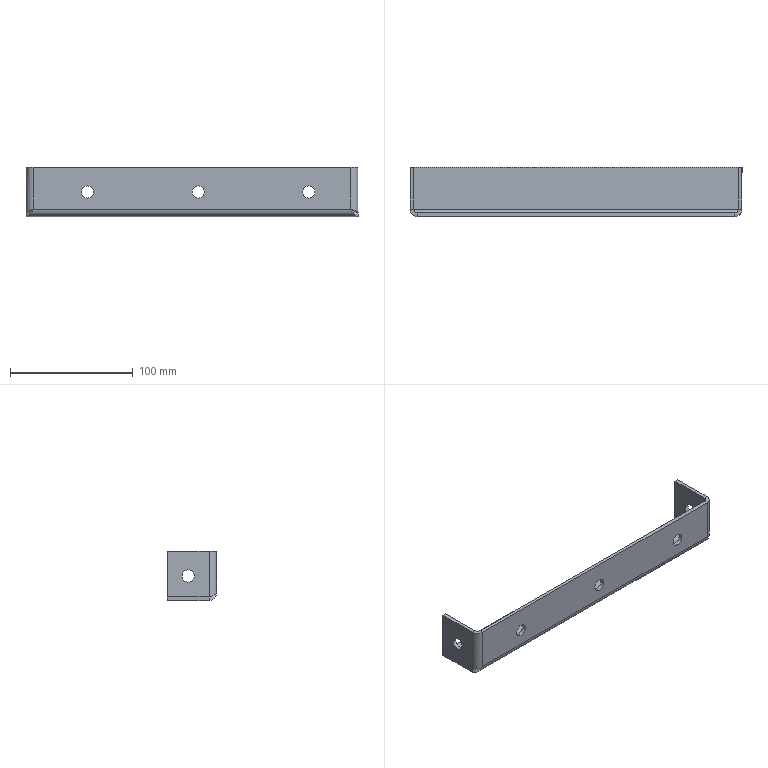Part | SolidWorks | features CornerFeat 1, EdgeFlange 1, FlatPattern 1, ICE 1, SMBaseFlange 1, SheetMetal 1 | 1 solid | 40 faces | box 270 x 40 x 40 mm | volume 67307 mm3 | plane 20 | cylinder 16 | spline 4 | commonest cylinder face diameters 10 x10 6 x3 12 x3
STEP:
#1=CARTESIAN_POINT('',(132.,28.,0.));
#2=VERTEX_POINT('',#1);
#3=CARTESIAN_POINT('',(132.,18.,0.));
#4=VERTEX_POINT('',#3);
#5=CARTESIAN_POINT('',(132.,23.,0.));
#6=DIRECTION('',(-1.,0.,0.));
#7=DIRECTION('',(0.,-1.,0.));
#8=AXIS2_PLACEMENT_3D('',#5,#6,#7);
#9=CIRCLE('',#8,5.);
#10=EDGE_CURVE('',#2,#4,#9,.T.);
#11=ORIENTED_EDGE('',*,*,#10,.T.);
#12=CARTESIAN_POINT('',(135.,18.,0.));
#13=VERTEX_POINT('',#12);
#14=CARTESIAN_POINT('',(-239.,18.,0.));
#15=DIRECTION('',(1.,0.,0.));
#16=VECTOR('',#15,1000.);
#17=LINE('',#14,#16);
#18=EDGE_CURVE('',#4,#13,#17,.T.);
#19=ORIENTED_EDGE('',*,*,#18,.T.);
#20=CARTESIAN_POINT('',(135.,28.,0.));
#21=VERTEX_POINT('',#20);
#22=CARTESIAN_POINT('',(135.,23.,0.));
#23=DIRECTION('',(1.,0.,0.));
#24=DIRECTION('',(0.,1.,0.));
#25=AXIS2_PLACEMENT_3D('',#22,#23,#24);
#26=CIRCLE('',#25,5.);
#27=EDGE_CURVE('',#13,#21,#26,.T.);
#28=ORIENTED_EDGE('',*,*,#27,.T.);
#29=CARTESIAN_POINT('',(-239.,28.,0.));
#30=DIRECTION('',(1.,0.,0.));
#31=VECTOR('',#30,1000.);
#32=LINE('',#29,#31);
#33=EDGE_CURVE('',#2,#21,#32,.T.);
#34=ORIENTED_EDGE('',*,*,#33,.F.);
#35=EDGE_LOOP('',(#11,#19,#28,#34));
#36=FACE_OUTER_BOUND('',#35,.T.);
#37=CARTESIAN_POINT('',(-239.,23.,0.));
#38=DIRECTION('',(1.,0.,0.));
#39=DIRECTION('',(0.,1.,0.));
#40=AXIS2_PLACEMENT_3D('',#37,#38,#39);
#41=CYLINDRICAL_SURFACE('',#40,5.);
#42=ADVANCED_FACE('',(#36),#41,.F.);
#43=CARTESIAN_POINT('',(-135.,18.,0.));
#44=VERTEX_POINT('',#43);
#45=CARTESIAN_POINT('',(-135.,28.,0.));
#46=VERTEX_POINT('',#45);
#47=CARTESIAN_POINT('',(-135.,23.,0.));
#48=DIRECTION('',(1.,0.,0.));
#49=DIRECTION('',(0.,1.,0.));
#50=AXIS2_PLACEMENT_3D('',#47,#48,#49);
#51=CIRCLE('',#50,5.);
#52=EDGE_CURVE('',#44,#46,#51,.T.);
#53=ORIENTED_EDGE('',*,*,#52,.F.);
#54=CARTESIAN_POINT('',(-132.,18.,0.));
#55=VERTEX_POINT('',#54);
#56=CARTESIAN_POINT('',(-239.,18.,0.));
#57=DIRECTION('',(1.,0.,0.));
#58=VECTOR('',#57,1000.);
#59=LINE('',#56,#58);
#60=EDGE_CURVE('',#44,#55,#59,.T.);
#61=ORIENTED_EDGE('',*,*,#60,.T.);
#62=CARTESIAN_POINT('',(-132.,28.,0.));
#63=VERTEX_POINT('',#62);
#64=CARTESIAN_POINT('',(-132.,23.,0.));
#65=DIRECTION('',(1.,0.,0.));
#66=DIRECTION('',(0.,1.,0.));
#67=AXIS2_PLACEMENT_3D('',#64,#65,#66);
#68=CIRCLE('',#67,5.);
#69=EDGE_CURVE('',#55,#63,#68,.T.);
#70=ORIENTED_EDGE('',*,*,#69,.T.);
#71=CARTESIAN_POINT('',(-239.,28.,0.));
#72=DIRECTION('',(1.,0.,0.));
#73=VECTOR('',#72,1000.);
#74=LINE('',#71,#73);
#75=EDGE_CURVE('',#46,#63,#74,.T.);
#76=ORIENTED_EDGE('',*,*,#75,.F.);
#77=EDGE_LOOP('',(#53,#61,#70,#76));
#78=FACE_OUTER_BOUND('',#77,.T.);
#79=CARTESIAN_POINT('',(-239.,23.,0.));
#80=DIRECTION('',(1.,0.,0.));
#81=DIRECTION('',(0.,1.,0.));
#82=AXIS2_PLACEMENT_3D('',#79,#80,#81);
#83=CYLINDRICAL_SURFACE('',#82,5.);
#84=ADVANCED_FACE('',(#78),#83,.F.);
#85=CARTESIAN_POINT('',(95.,3.,-5.));
#86=VERTEX_POINT('',#85);
#87=CARTESIAN_POINT('',(95.,3.,5.));
#88=VERTEX_POINT('',#87);
#89=CARTESIAN_POINT('',(95.,3.,0.));
#90=DIRECTION('',(0.,1.,0.));
#91=DIRECTION('',(0.,0.,1.));
#92=AXIS2_PLACEMENT_3D('',#89,#90,#91);
#93=CIRCLE('',#92,5.);
#94=EDGE_CURVE('',#86,#88,#93,.T.);
#95=ORIENTED_EDGE('',*,*,#94,.T.);
#96=CARTESIAN_POINT('',(95.,0.,5.));
#97=VERTEX_POINT('',#96);
#98=CARTESIAN_POINT('',(95.,3.,5.));
#99=DIRECTION('',(0.,-1.,0.));
#100=VECTOR('',#99,1000.);
#101=LINE('',#98,#100);
#102=EDGE_CURVE('',#88,#97,#101,.T.);
#103=ORIENTED_EDGE('',*,*,#102,.T.);
#104=CARTESIAN_POINT('',(95.,0.,-5.));
#105=VERTEX_POINT('',#104);
#106=CARTESIAN_POINT('',(95.,0.,0.));
#107=DIRECTION('',(0.,1.,0.));
#108=DIRECTION('',(0.,0.,1.));
#109=AXIS2_PLACEMENT_3D('',#106,#107,#108);
#110=CIRCLE('',#109,5.);
#111=EDGE_CURVE('',#105,#97,#110,.T.);
#112=ORIENTED_EDGE('',*,*,#111,.F.);
#113=CARTESIAN_POINT('',(95.,3.,-5.));
#114=DIRECTION('',(0.,-1.,0.));
#115=VECTOR('',#114,1000.);
#116=LINE('',#113,#115);
#117=EDGE_CURVE('',#86,#105,#116,.T.);
#118=ORIENTED_EDGE('',*,*,#117,.F.);
#119=EDGE_LOOP('',(#95,#103,#112,#118));
#120=FACE_OUTER_BOUND('',#119,.T.);
#121=CARTESIAN_POINT('',(95.,3.,0.));
#122=DIRECTION('',(0.,-1.,0.));
#123=DIRECTION('',(0.,0.,-1.));
#124=AXIS2_PLACEMENT_3D('',#121,#122,#123);
#125=CYLINDRICAL_SURFACE('',#124,5.);
#126=ADVANCED_FACE('',(#120),#125,.F.);
#127=CARTESIAN_POINT('',(5.,3.,-5.));
#128=VERTEX_POINT('',#127);
#129=CARTESIAN_POINT('',(5.,3.,5.));
#130=VERTEX_POINT('',#129);
#131=CARTESIAN_POINT('',(5.,3.,0.));
#132=DIRECTION('',(0.,1.,0.));
#133=DIRECTION('',(0.,0.,1.));
#134=AXIS2_PLACEMENT_3D('',#131,#132,#133);
#135=CIRCLE('',#134,5.);
#136=EDGE_CURVE('',#128,#130,#135,.T.);
#137=ORIENTED_EDGE('',*,*,#136,.T.);
#138=CARTESIAN_POINT('',(5.,0.,5.));
#139=VERTEX_POINT('',#138);
#140=CARTESIAN_POINT('',(5.,3.,5.));
#141=DIRECTION('',(0.,-1.,0.));
#142=VECTOR('',#141,1000.);
#143=LINE('',#140,#142);
#144=EDGE_CURVE('',#130,#139,#143,.T.);
#145=ORIENTED_EDGE('',*,*,#144,.T.);
#146=CARTESIAN_POINT('',(5.,0.,-5.));
#147=VERTEX_POINT('',#146);
#148=CARTESIAN_POINT('',(5.,0.,0.));
#149=DIRECTION('',(0.,1.,0.));
#150=DIRECTION('',(0.,0.,1.));
#151=AXIS2_PLACEMENT_3D('',#148,#149,#150);
#152=CIRCLE('',#151,5.);
#153=EDGE_CURVE('',#147,#139,#152,.T.);
#154=ORIENTED_EDGE('',*,*,#153,.F.);
#155=CARTESIAN_POINT('',(5.,3.,-5.));
#156=DIRECTION('',(0.,-1.,0.));
#157=VECTOR('',#156,1000.);
#158=LINE('',#155,#157);
#159=EDGE_CURVE('',#128,#147,#158,.T.);
#160=ORIENTED_EDGE('',*,*,#159,.F.);
#161=EDGE_LOOP('',(#137,#145,#154,#160));
#162=FACE_OUTER_BOUND('',#161,.T.);
#163=CARTESIAN_POINT('',(5.,3.,0.));
#164=DIRECTION('',(0.,-1.,0.));
#165=DIRECTION('',(0.,0.,-1.));
#166=AXIS2_PLACEMENT_3D('',#163,#164,#165);
#167=CYLINDRICAL_SURFACE('',#166,5.);
#168=ADVANCED_FACE('',(#162),#167,.F.);
#169=CARTESIAN_POINT('',(-85.,3.,-5.));
#170=VERTEX_POINT('',#169);
#171=CARTESIAN_POINT('',(-85.,3.,5.));
#172=VERTEX_POINT('',#171);
#173=CARTESIAN_POINT('',(-85.,3.,0.));
#174=DIRECTION('',(0.,1.,0.));
#175=DIRECTION('',(0.,0.,1.));
#176=AXIS2_PLACEMENT_3D('',#173,#174,#175);
#177=CIRCLE('',#176,5.);
#178=EDGE_CURVE('',#170,#172,#177,.T.);
#179=ORIENTED_EDGE('',*,*,#178,.T.);
#180=CARTESIAN_POINT('',(-85.,0.,5.));
#181=VERTEX_POINT('',#180);
#182=CARTESIAN_POINT('',(-85.,3.,5.));
#183=DIRECTION('',(0.,-1.,0.));
#184=VECTOR('',#183,1000.);
#185=LINE('',#182,#184);
#186=EDGE_CURVE('',#172,#181,#185,.T.);
#187=ORIENTED_EDGE('',*,*,#186,.T.);
#188=CARTESIAN_POINT('',(-85.,0.,-5.));
#189=VERTEX_POINT('',#188);
#190=CARTESIAN_POINT('',(-85.,0.,0.));
#191=DIRECTION('',(0.,1.,0.));
#192=DIRECTION('',(0.,0.,1.));
#193=AXIS2_PLACEMENT_3D('',#190,#191,#192);
#194=CIRCLE('',#193,5.);
#195=EDGE_CURVE('',#189,#181,#194,.T.);
#196=ORIENTED_EDGE('',*,*,#195,.F.);
#197=CARTESIAN_POINT('',(-85.,3.,-5.));
#198=DIRECTION('',(0.,-1.,0.));
#199=VECTOR('',#198,1000.);
#200=LINE('',#197,#199);
#201=EDGE_CURVE('',#170,#189,#200,.T.);
#202=ORIENTED_EDGE('',*,*,#201,.F.);
#203=EDGE_LOOP('',(#179,#187,#196,#202));
#204=FACE_OUTER_BOUND('',#203,.T.);
#205=CARTESIAN_POINT('',(-85.,3.,0.));
#206=DIRECTION('',(0.,-1.,0.));
#207=DIRECTION('',(0.,0.,-1.));
#208=AXIS2_PLACEMENT_3D('',#205,#206,#207);
#209=CYLINDRICAL_SURFACE('',#208,5.);
#210=ADVANCED_FACE('',(#204),#209,.F.);
#211=ORIENTED_EDGE('',*,*,#136,.F.);
#212=CARTESIAN_POINT('',(5.,3.,0.));
#213=DIRECTION('',(0.,1.,0.));
#214=DIRECTION('',(0.,0.,1.));
#215=AXIS2_PLACEMENT_3D('',#212,#213,#214);
#216=CIRCLE('',#215,5.);
#217=EDGE_CURVE('',#130,#128,#216,.T.);
#218=ORIENTED_EDGE('',*,*,#217,.F.);
#219=EDGE_LOOP('',(#211,#218));
#220=FACE_BOUND('',#219,.T.);
#221=ORIENTED_EDGE('',*,*,#178,.F.);
#222=CARTESIAN_POINT('',(-85.,3.,0.));
#223=DIRECTION('',(0.,1.,0.));
#224=DIRECTION('',(0.,0.,1.));
#225=AXIS2_PLACEMENT_3D('',#222,#223,#224);
#226=CIRCLE('',#225,5.);
#227=EDGE_CURVE('',#172,#170,#226,.T.);
#228=ORIENTED_EDGE('',*,*,#227,.F.);
#229=EDGE_LOOP('',(#221,#228));
#230=FACE_BOUND('',#229,.T.);
#231=ORIENTED_EDGE('',*,*,#94,.F.);
#232=CARTESIAN_POINT('',(95.,3.,0.));
#233=DIRECTION('',(0.,1.,0.));
#234=DIRECTION('',(0.,0.,1.));
#235=AXIS2_PLACEMENT_3D('',#232,#233,#234);
#236=CIRCLE('',#235,5.);
#237=EDGE_CURVE('',#88,#86,#236,.T.);
#238=ORIENTED_EDGE('',*,*,#237,.F.);
#239=EDGE_LOOP('',(#231,#238));
#240=FACE_BOUND('',#239,.T.);
#241=CARTESIAN_POINT('',(-129.,3.,-14.));
#242=VERTEX_POINT('',#241);
#243=CARTESIAN_POINT('',(129.,3.,-14.));
#244=VERTEX_POINT('',#243);
#245=CARTESIAN_POINT('',(-131.293,3.,-14.));
#246=DIRECTION('',(1.,0.,0.));
#247=VECTOR('',#246,1000.);
#248=LINE('',#245,#247);
#249=EDGE_CURVE('',#242,#244,#248,.T.);
#250=ORIENTED_EDGE('',*,*,#249,.F.);
#251=CARTESIAN_POINT('',(-129.,3.,20.));
#252=VERTEX_POINT('',#251);
#253=CARTESIAN_POINT('',(-129.,3.,20.));
#254=DIRECTION('',(0.,0.,-1.));
#255=VECTOR('',#254,1000.);
#256=LINE('',#253,#255);
#257=EDGE_CURVE('',#252,#242,#256,.T.);
#258=ORIENTED_EDGE('',*,*,#257,.F.);
#259=CARTESIAN_POINT('',(129.,3.,20.));
#260=VERTEX_POINT('',#259);
#261=CARTESIAN_POINT('',(-135.,3.,20.));
#262=DIRECTION('',(1.,0.,0.));
#263=VECTOR('',#262,1000.);
#264=LINE('',#261,#263);
#265=EDGE_CURVE('',#252,#260,#264,.T.);
#266=ORIENTED_EDGE('',*,*,#265,.T.);
#267=CARTESIAN_POINT('',(129.,3.,-16.293));
#268=DIRECTION('',(0.,0.,1.));
#269=VECTOR('',#268,1000.);
#270=LINE('',#267,#269);
#271=EDGE_CURVE('',#244,#260,#270,.T.);
#272=ORIENTED_EDGE('',*,*,#271,.F.);
#273=EDGE_LOOP('',(#250,#258,#266,#272));
#274=FACE_OUTER_BOUND('',#273,.T.);
#275=CARTESIAN_POINT('',(0.,3.,0.));
#276=DIRECTION('',(0.,1.,0.));
#277=DIRECTION('',(0.,0.,1.));
#278=AXIS2_PLACEMENT_3D('',#275,#276,#277);
#279=PLANE('',#278);
#280=ADVANCED_FACE('',(#220,#230,#240,#274),#279,.T.);
#281=ORIENTED_EDGE('',*,*,#111,.T.);
#282=CARTESIAN_POINT('',(95.,0.,0.));
#283=DIRECTION('',(0.,1.,0.));
#284=DIRECTION('',(0.,0.,1.));
#285=AXIS2_PLACEMENT_3D('',#282,#283,#284);
#286=CIRCLE('',#285,5.);
#287=EDGE_CURVE('',#97,#105,#286,.T.);
#288=ORIENTED_EDGE('',*,*,#287,.T.);
#289=EDGE_LOOP('',(#281,#288));
#290=FACE_BOUND('',#289,.T.);
#291=ORIENTED_EDGE('',*,*,#153,.T.);
#292=CARTESIAN_POINT('',(5.,0.,0.));
#293=DIRECTION('',(0.,1.,0.));
#294=DIRECTION('',(0.,0.,1.));
#295=AXIS2_PLACEMENT_3D('',#292,#293,#294);
#296=CIRCLE('',#295,5.);
#297=EDGE_CURVE('',#139,#147,#296,.T.);
#298=ORIENTED_EDGE('',*,*,#297,.T.);
#299=EDGE_LOOP('',(#291,#298));
#300=FACE_BOUND('',#299,.T.);
#301=ORIENTED_EDGE('',*,*,#195,.T.);
#302=CARTESIAN_POINT('',(-85.,0.,0.));
#303=DIRECTION('',(0.,1.,0.));
#304=DIRECTION('',(0.,0.,1.));
#305=AXIS2_PLACEMENT_3D('',#302,#303,#304);
#306=CIRCLE('',#305,5.);
#307=EDGE_CURVE('',#181,#189,#306,.T.);
#308=ORIENTED_EDGE('',*,*,#307,.T.);
#309=EDGE_LOOP('',(#301,#308));
#310=FACE_BOUND('',#309,.T.);
#311=CARTESIAN_POINT('',(-129.,0.,20.));
#312=VERTEX_POINT('',#311);
#313=CARTESIAN_POINT('',(-129.,0.,-14.));
#314=VERTEX_POINT('',#313);
#315=CARTESIAN_POINT('',(-129.,0.,20.));
#316=DIRECTION('',(0.,0.,-1.));
#317=VECTOR('',#316,1000.);
#318=LINE('',#315,#317);
#319=EDGE_CURVE('',#312,#314,#318,.T.);
#320=ORIENTED_EDGE('',*,*,#319,.T.);
#321=CARTESIAN_POINT('',(129.,0.,-14.));
#322=VERTEX_POINT('',#321);
#323=CARTESIAN_POINT('',(-131.293,0.,-14.));
#324=DIRECTION('',(1.,0.,0.));
#325=VECTOR('',#324,1000.);
#326=LINE('',#323,#325);
#327=EDGE_CURVE('',#314,#322,#326,.T.);
#328=ORIENTED_EDGE('',*,*,#327,.T.);
#329=CARTESIAN_POINT('',(129.,0.,20.));
#330=VERTEX_POINT('',#329);
#331=CARTESIAN_POINT('',(129.,0.,-16.293));
#332=DIRECTION('',(0.,0.,1.));
#333=VECTOR('',#332,1000.);
#334=LINE('',#331,#333);
#335=EDGE_CURVE('',#322,#330,#334,.T.);
#336=ORIENTED_EDGE('',*,*,#335,.T.);
#337=CARTESIAN_POINT('',(-135.,0.,20.));
#338=DIRECTION('',(1.,0.,0.));
#339=VECTOR('',#338,1000.);
#340=LINE('',#337,#339);
#341=EDGE_CURVE('',#312,#330,#340,.T.);
#342=ORIENTED_EDGE('',*,*,#341,.F.);
#343=EDGE_LOOP('',(#320,#328,#336,#342));
#344=FACE_OUTER_BOUND('',#343,.T.);
#345=CARTESIAN_POINT('',(0.,0.,0.));
#346=DIRECTION('',(0.,1.,0.));
#347=DIRECTION('',(0.,0.,1.));
#348=AXIS2_PLACEMENT_3D('',#345,#346,#347);
#349=PLANE('',#348);
#350=ADVANCED_FACE('',(#290,#300,#310,#344),#349,.F.);
#351=CARTESIAN_POINT('',(-129.,3.,20.));
#352=DIRECTION('',(0.,-1.,0.));
#353=VECTOR('',#352,1000.);
#354=LINE('',#351,#353);
#355=EDGE_CURVE('',#252,#312,#354,.T.);
#356=ORIENTED_EDGE('',*,*,#355,.T.);
#357=ORIENTED_EDGE('',*,*,#341,.T.);
#358=CARTESIAN_POINT('',(129.,3.,20.));
#359=DIRECTION('',(0.,-1.,0.));
#360=VECTOR('',#359,1000.);
#361=LINE('',#358,#360);
#362=EDGE_CURVE('',#260,#330,#361,.T.);
#363=ORIENTED_EDGE('',*,*,#362,.F.);
#364=ORIENTED_EDGE('',*,*,#265,.F.);
#365=EDGE_LOOP('',(#356,#357,#363,#364));
#366=FACE_OUTER_BOUND('',#365,.T.);
#367=CARTESIAN_POINT('',(-135.,3.,20.));
#368=DIRECTION('',(0.,0.,-1.));
#369=DIRECTION('',(-1.,0.,0.));
#370=AXIS2_PLACEMENT_3D('',#367,#368,#369);
#371=PLANE('',#370);
#372=ADVANCED_FACE('',(#366),#371,.F.);
#373=ORIENTED_EDGE('',*,*,#186,.F.);
#374=ORIENTED_EDGE('',*,*,#227,.T.);
#375=ORIENTED_EDGE('',*,*,#201,.T.);
#376=ORIENTED_EDGE('',*,*,#307,.F.);
#377=EDGE_LOOP('',(#373,#374,#375,#376));
#378=FACE_OUTER_BOUND('',#377,.T.);
#379=CARTESIAN_POINT('',(-85.,3.,0.));
#380=DIRECTION('',(0.,-1.,0.));
#381=DIRECTION('',(0.,0.,-1.));
#382=AXIS2_PLACEMENT_3D('',#379,#380,#381);
#383=CYLINDRICAL_SURFACE('',#382,5.);
#384=ADVANCED_FACE('',(#378),#383,.F.);
#385=ORIENTED_EDGE('',*,*,#144,.F.);
#386=ORIENTED_EDGE('',*,*,#217,.T.);
#387=ORIENTED_EDGE('',*,*,#159,.T.);
#388=ORIENTED_EDGE('',*,*,#297,.F.);
#389=EDGE_LOOP('',(#385,#386,#387,#388));
#390=FACE_OUTER_BOUND('',#389,.T.);
#391=CARTESIAN_POINT('',(5.,3.,0.));
#392=DIRECTION('',(0.,-1.,0.));
#393=DIRECTION('',(0.,0.,-1.));
#394=AXIS2_PLACEMENT_3D('',#391,#392,#393);
#395=CYLINDRICAL_SURFACE('',#394,5.);
#396=ADVANCED_FACE('',(#390),#395,.F.);
#397=ORIENTED_EDGE('',*,*,#102,.F.);
#398=ORIENTED_EDGE('',*,*,#237,.T.);
#399=ORIENTED_EDGE('',*,*,#117,.T.);
#400=ORIENTED_EDGE('',*,*,#287,.F.);
#401=EDGE_LOOP('',(#397,#398,#399,#400));
#402=FACE_OUTER_BOUND('',#401,.T.);
#403=CARTESIAN_POINT('',(95.,3.,0.));
#404=DIRECTION('',(0.,-1.,0.));
#405=DIRECTION('',(0.,0.,-1.));
#406=AXIS2_PLACEMENT_3D('',#403,#404,#405);
#407=CYLINDRICAL_SURFACE('',#406,5.);
#408=ADVANCED_FACE('',(#402),#407,.F.);
#409=CARTESIAN_POINT('',(-132.,6.,20.));
#410=VERTEX_POINT('',#409);
#411=CARTESIAN_POINT('',(-135.,6.,20.));
#412=VERTEX_POINT('',#411);
#413=CARTESIAN_POINT('',(-132.,6.,20.));
#414=DIRECTION('',(-1.,0.,0.));
#415=VECTOR('',#414,1000.);
#416=LINE('',#413,#415);
#417=EDGE_CURVE('',#410,#412,#416,.T.);
#418=ORIENTED_EDGE('',*,*,#417,.T.);
#419=CARTESIAN_POINT('',(-129.,6.,20.));
#420=DIRECTION('',(0.,0.,1.));
#421=DIRECTION('',(1.,0.,0.));
#422=AXIS2_PLACEMENT_3D('',#419,#420,#421);
#423=CIRCLE('',#422,6.);
#424=EDGE_CURVE('',#412,#312,#423,.T.);
#425=ORIENTED_EDGE('',*,*,#424,.T.);
#426=ORIENTED_EDGE('',*,*,#355,.F.);
#427=CARTESIAN_POINT('',(-129.,6.,20.));
#428=DIRECTION('',(0.,0.,1.));
#429=DIRECTION('',(1.,0.,0.));
#430=AXIS2_PLACEMENT_3D('',#427,#428,#429);
#431=CIRCLE('',#430,3.);
#432=EDGE_CURVE('',#410,#252,#431,.T.);
#433=ORIENTED_EDGE('',*,*,#432,.F.);
#434=EDGE_LOOP('',(#418,#425,#426,#433));
#435=FACE_OUTER_BOUND('',#434,.T.);
#436=CARTESIAN_POINT('',(-129.,6.,20.));
#437=DIRECTION('',(0.,0.,-1.));
#438=DIRECTION('',(-1.,0.,0.));
#439=AXIS2_PLACEMENT_3D('',#436,#437,#438);
#440=PLANE('',#439);
#441=ADVANCED_FACE('',(#435),#440,.F.);
#442=CARTESIAN_POINT('',(-135.,6.,-16.9));
#443=VERTEX_POINT('',#442);
#444=CARTESIAN_POINT('',(-129.,0.,-14.));
#445=CARTESIAN_POINT('',(-129.396,0.,-14.122));
#446=CARTESIAN_POINT('',(-129.786,0.03889,-14.242));
#447=CARTESIAN_POINT('',(-130.361,0.1531,-14.422));
#448=CARTESIAN_POINT('',(-130.551,0.2005,-14.482));
#449=CARTESIAN_POINT('',(-130.927,0.3144,-14.603));
#450=CARTESIAN_POINT('',(-131.114,0.3813,-14.664));
#451=CARTESIAN_POINT('',(-131.66,0.6074,-14.846));
#452=CARTESIAN_POINT('',(-132.005,0.7918,-14.966));
#453=CARTESIAN_POINT('',(-132.655,1.226,-15.207));
#454=CARTESIAN_POINT('',(-132.964,1.479,-15.329));
#455=CARTESIAN_POINT('',(-133.519,2.033,-15.57));
#456=CARTESIAN_POINT('',(-133.767,2.335,-15.69));
#457=CARTESIAN_POINT('',(-134.204,2.987,-15.931));
#458=CARTESIAN_POINT('',(-134.392,3.339,-16.053));
#459=CARTESIAN_POINT('',(-134.692,4.062,-16.294));
#460=CARTESIAN_POINT('',(-134.806,4.435,-16.414));
#461=CARTESIAN_POINT('',(-134.961,5.208,-16.656));
#462=CARTESIAN_POINT('',(-135.,5.604,-16.778));
#463=CARTESIAN_POINT('',(-135.,6.,-16.9));
#464=B_SPLINE_CURVE_WITH_KNOTS('',3,(#444,#445,#446,#447,#448,#449,#450,#451,#452,#453,#454,#455,#456,#457,#458,#459,#460,#461,#462,#463),.UNSPECIFIED.,.F.,.F.,(4,2,2,2,2,2,2,2,2,4),(0.,0.001226,0.001839,0.002452,0.003677,0.004903,0.006129,0.007355,0.008581,0.009807),.UNSPECIFIED.);
#465=EDGE_CURVE('',#314,#443,#464,.T.);
#466=ORIENTED_EDGE('',*,*,#465,.T.);
#467=CARTESIAN_POINT('',(-132.,6.,-16.9));
#468=VERTEX_POINT('',#467);
#469=CARTESIAN_POINT('',(-132.,6.,-16.9));
#470=CARTESIAN_POINT('',(-133.,6.,-16.9));
#471=CARTESIAN_POINT('',(-134.,6.,-16.9));
#472=CARTESIAN_POINT('',(-135.,6.,-16.9));
#473=B_SPLINE_CURVE_WITH_KNOTS('',3,(#469,#470,#471,#472),.UNSPECIFIED.,.F.,.F.,(4,4),(0.,1.),.UNSPECIFIED.);
#474=EDGE_CURVE('',#468,#443,#473,.T.);
#475=ORIENTED_EDGE('',*,*,#474,.F.);
#476=CARTESIAN_POINT('',(-129.,3.,-14.));
#477=CARTESIAN_POINT('',(-129.396,3.,-14.244));
#478=CARTESIAN_POINT('',(-129.781,3.077,-14.48));
#479=CARTESIAN_POINT('',(-130.327,3.302,-14.844));
#480=CARTESIAN_POINT('',(-130.502,3.396,-14.966));
#481=CARTESIAN_POINT('',(-130.828,3.613,-15.207));
#482=CARTESIAN_POINT('',(-130.979,3.737,-15.327));
#483=CARTESIAN_POINT('',(-131.258,4.015,-15.569));
#484=CARTESIAN_POINT('',(-131.385,4.169,-15.691));
#485=CARTESIAN_POINT('',(-131.602,4.494,-15.932));
#486=CARTESIAN_POINT('',(-131.695,4.667,-16.052));
#487=CARTESIAN_POINT('',(-131.846,5.031,-16.294));
#488=CARTESIAN_POINT('',(-131.904,5.221,-16.416));
#489=CARTESIAN_POINT('',(-131.98,5.606,-16.657));
#490=CARTESIAN_POINT('',(-132.,5.802,-16.778));
#491=CARTESIAN_POINT('',(-132.,6.,-16.9));
#492=B_SPLINE_CURVE_WITH_KNOTS('',3,(#476,#477,#478,#479,#480,#481,#482,#483,#484,#485,#486,#487,#488,#489,#490,#491),.UNSPECIFIED.,.F.,.F.,(4,2,2,2,2,2,2,4),(0.,0.001373,0.002059,0.002745,0.003432,0.004118,0.004804,0.005491),.UNSPECIFIED.);
#493=EDGE_CURVE('',#242,#468,#492,.T.);
#494=ORIENTED_EDGE('',*,*,#493,.F.);
#495=CARTESIAN_POINT('',(-129.,0.,-14.));
#496=CARTESIAN_POINT('',(-129.,3.,-14.));
#497=B_SPLINE_CURVE_WITH_KNOTS('',1,(#495,#496),.UNSPECIFIED.,.F.,.F.,(2,2),(0.,1.),.UNSPECIFIED.);
#498=EDGE_CURVE('',#314,#242,#497,.T.);
#499=ORIENTED_EDGE('',*,*,#498,.F.);
#500=EDGE_LOOP('',(#466,#475,#494,#499));
#501=FACE_OUTER_BOUND('',#500,.T.);
#502=CARTESIAN_POINT('',(-129.,-0.03,-14.));
#503=CARTESIAN_POINT('',(-129.789,-0.03,-14.242));
#504=CARTESIAN_POINT('',(-130.578,0.1269,-14.483));
#505=CARTESIAN_POINT('',(-132.037,0.7311,-14.967));
#506=CARTESIAN_POINT('',(-132.706,1.178,-15.208));
#507=CARTESIAN_POINT('',(-133.822,2.294,-15.692));
#508=CARTESIAN_POINT('',(-134.269,2.963,-15.933));
#509=CARTESIAN_POINT('',(-134.873,4.422,-16.417));
#510=CARTESIAN_POINT('',(-135.03,5.211,-16.658));
#511=CARTESIAN_POINT('',(-135.03,6.,-16.9));
#512=CARTESIAN_POINT('',(-129.,0.,-14.));
#513=CARTESIAN_POINT('',(-129.786,0.,-14.242));
#514=CARTESIAN_POINT('',(-130.57,0.1562,-14.483));
#515=CARTESIAN_POINT('',(-132.022,0.7573,-14.967));
#516=CARTESIAN_POINT('',(-132.687,1.202,-15.208));
#517=CARTESIAN_POINT('',(-133.798,2.313,-15.692));
#518=CARTESIAN_POINT('',(-134.243,2.978,-15.933));
#519=CARTESIAN_POINT('',(-134.844,4.43,-16.417));
#520=CARTESIAN_POINT('',(-135.,5.214,-16.658));
#521=CARTESIAN_POINT('',(-135.,6.,-16.9));
#522=CARTESIAN_POINT('',(-129.,3.,-14.));
#523=CARTESIAN_POINT('',(-129.393,3.,-14.242));
#524=CARTESIAN_POINT('',(-129.785,3.078,-14.483));
#525=CARTESIAN_POINT('',(-130.511,3.379,-14.967));
#526=CARTESIAN_POINT('',(-130.844,3.601,-15.208));
#527=CARTESIAN_POINT('',(-131.399,4.156,-15.692));
#528=CARTESIAN_POINT('',(-131.621,4.489,-15.933));
#529=CARTESIAN_POINT('',(-131.922,5.215,-16.417));
#530=CARTESIAN_POINT('',(-132.,5.607,-16.658));
#531=CARTESIAN_POINT('',(-132.,6.,-16.9));
#532=CARTESIAN_POINT('',(-129.,3.03,-14.));
#533=CARTESIAN_POINT('',(-129.389,3.03,-14.242));
#534=CARTESIAN_POINT('',(-129.777,3.108,-14.483));
#535=CARTESIAN_POINT('',(-130.496,3.405,-14.967));
#536=CARTESIAN_POINT('',(-130.825,3.625,-15.208));
#537=CARTESIAN_POINT('',(-131.375,4.175,-15.692));
#538=CARTESIAN_POINT('',(-131.595,4.504,-15.933));
#539=CARTESIAN_POINT('',(-131.892,5.223,-16.417));
#540=CARTESIAN_POINT('',(-131.97,5.611,-16.658));
#541=CARTESIAN_POINT('',(-131.97,6.,-16.9));
#542=B_SPLINE_SURFACE_WITH_KNOTS('',1,3,((#502,#503,#504,#505,#506,#507,#508,#509,#510,#511),(#512,#513,#514,#515,#516,#517,#518,#519,#520,#521),(#522,#523,#524,#525,#526,#527,#528,#529,#530,#531),(#532,#533,#534,#535,#536,#537,#538,#539,#540,#541)),.UNSPECIFIED.,.F.,.F.,.F.,(2,1,1,2),(4,2,2,2,4),(-0.01,0.,1.,1.01),(0.,0.25,0.5,0.75,1.),.UNSPECIFIED.);
#543=ADVANCED_FACE('',(#501),#542,.F.);
#544=ORIENTED_EDGE('',*,*,#257,.T.);
#545=ORIENTED_EDGE('',*,*,#493,.T.);
#546=CARTESIAN_POINT('',(-132.,6.,-20.));
#547=DIRECTION('',(0.,0.,1.));
#548=VECTOR('',#547,1000.);
#549=LINE('',#546,#548);
#550=EDGE_CURVE('',#468,#410,#549,.T.);
#551=ORIENTED_EDGE('',*,*,#550,.T.);
#552=ORIENTED_EDGE('',*,*,#432,.T.);
#553=EDGE_LOOP('',(#544,#545,#551,#552));
#554=FACE_OUTER_BOUND('',#553,.T.);
#555=CARTESIAN_POINT('',(-129.,6.,-34.691));
#556=DIRECTION('',(0.,0.,1.));
#557=DIRECTION('',(1.,0.,0.));
#558=AXIS2_PLACEMENT_3D('',#555,#556,#557);
#559=CYLINDRICAL_SURFACE('',#558,3.);
#560=ADVANCED_FACE('',(#554),#559,.F.);
#561=ORIENTED_EDGE('',*,*,#319,.F.);
#562=ORIENTED_EDGE('',*,*,#424,.F.);
#563=CARTESIAN_POINT('',(-135.,6.,-20.));
#564=DIRECTION('',(0.,0.,-1.));
#565=VECTOR('',#564,1000.);
#566=LINE('',#563,#565);
#567=EDGE_CURVE('',#412,#443,#566,.T.);
#568=ORIENTED_EDGE('',*,*,#567,.T.);
#569=ORIENTED_EDGE('',*,*,#465,.F.);
#570=EDGE_LOOP('',(#561,#562,#568,#569));
#571=FACE_OUTER_BOUND('',#570,.T.);
#572=CARTESIAN_POINT('',(-129.,6.,-34.691));
#573=DIRECTION('',(0.,0.,1.));
#574=DIRECTION('',(1.,0.,0.));
#575=AXIS2_PLACEMENT_3D('',#572,#573,#574);
#576=CYLINDRICAL_SURFACE('',#575,6.);
#577=ADVANCED_FACE('',(#571),#576,.T.);
#578=CARTESIAN_POINT('',(-132.,40.,20.));
#579=VERTEX_POINT('',#578);
#580=CARTESIAN_POINT('',(-132.,40.,-16.9));
#581=VERTEX_POINT('',#580);
#582=CARTESIAN_POINT('',(-132.,40.,-20.));
#583=DIRECTION('',(0.,0.,-1.));
#584=VECTOR('',#583,1000.);
#585=LINE('',#582,#584);
#586=EDGE_CURVE('',#579,#581,#585,.T.);
#587=ORIENTED_EDGE('',*,*,#586,.T.);
#588=CARTESIAN_POINT('',(-135.,40.,-16.9));
#589=VERTEX_POINT('',#588);
#590=CARTESIAN_POINT('',(-132.,40.,-16.9));
#591=DIRECTION('',(-1.,0.,0.));
#592=VECTOR('',#591,1000.);
#593=LINE('',#590,#592);
#594=EDGE_CURVE('',#581,#589,#593,.T.);
#595=ORIENTED_EDGE('',*,*,#594,.T.);
#596=CARTESIAN_POINT('',(-135.,40.,20.));
#597=VERTEX_POINT('',#596);
#598=CARTESIAN_POINT('',(-135.,40.,0.));
#599=DIRECTION('',(0.,0.,-1.));
#600=VECTOR('',#599,1000.);
#601=LINE('',#598,#600);
#602=EDGE_CURVE('',#597,#589,#601,.T.);
#603=ORIENTED_EDGE('',*,*,#602,.F.);
#604=CARTESIAN_POINT('',(-135.,40.,20.));
#605=DIRECTION('',(1.,0.,0.));
#606=VECTOR('',#605,1000.);
#607=LINE('',#604,#606);
#608=EDGE_CURVE('',#597,#579,#607,.T.);
#609=ORIENTED_EDGE('',*,*,#608,.T.);
#610=EDGE_LOOP('',(#587,#595,#603,#609));
#611=FACE_OUTER_BOUND('',#610,.T.);
#612=CARTESIAN_POINT('',(-135.,40.,-20.));
#613=DIRECTION('',(0.,-1.,0.));
#614=DIRECTION('',(1.,0.,0.));
#615=AXIS2_PLACEMENT_3D('',#612,#613,#614);
#616=PLANE('',#615);
#617=ADVANCED_FACE('',(#611),#616,.F.);
#618=ORIENTED_EDGE('',*,*,#60,.F.);
#619=CARTESIAN_POINT('',(-135.,23.,0.));
#620=DIRECTION('',(1.,0.,0.));
#621=DIRECTION('',(0.,1.,0.));
#622=AXIS2_PLACEMENT_3D('',#619,#620,#621);
#623=CIRCLE('',#622,5.);
#624=EDGE_CURVE('',#46,#44,#623,.T.);
#625=ORIENTED_EDGE('',*,*,#624,.F.);
#626=ORIENTED_EDGE('',*,*,#75,.T.);
#627=CARTESIAN_POINT('',(-132.,23.,0.));
#628=DIRECTION('',(1.,0.,0.));
#629=DIRECTION('',(0.,1.,0.));
#630=AXIS2_PLACEMENT_3D('',#627,#628,#629);
#631=CIRCLE('',#630,5.);
#632=EDGE_CURVE('',#63,#55,#631,.T.);
#633=ORIENTED_EDGE('',*,*,#632,.T.);
#634=EDGE_LOOP('',(#618,#625,#626,#633));
#635=FACE_OUTER_BOUND('',#634,.T.);
#636=CARTESIAN_POINT('',(-239.,23.,0.));
#637=DIRECTION('',(1.,0.,0.));
#638=DIRECTION('',(0.,1.,0.));
#639=AXIS2_PLACEMENT_3D('',#636,#637,#638);
#640=CYLINDRICAL_SURFACE('',#639,5.);
#641=ADVANCED_FACE('',(#635),#640,.F.);
#642=ORIENTED_EDGE('',*,*,#632,.F.);
#643=ORIENTED_EDGE('',*,*,#69,.F.);
#644=EDGE_LOOP('',(#642,#643));
#645=FACE_BOUND('',#644,.T.);
#646=ORIENTED_EDGE('',*,*,#550,.F.);
#647=CARTESIAN_POINT('',(-132.,6.,-16.9));
#648=DIRECTION('',(0.,1.,0.));
#649=VECTOR('',#648,1000.);
#650=LINE('',#647,#649);
#651=EDGE_CURVE('',#468,#581,#650,.T.);
#652=ORIENTED_EDGE('',*,*,#651,.T.);
#653=ORIENTED_EDGE('',*,*,#586,.F.);
#654=CARTESIAN_POINT('',(-132.,40.,20.));
#655=DIRECTION('',(0.,1.,0.));
#656=VECTOR('',#655,1000.);
#657=LINE('',#654,#656);
#658=EDGE_CURVE('',#410,#579,#657,.T.);
#659=ORIENTED_EDGE('',*,*,#658,.F.);
#660=EDGE_LOOP('',(#646,#652,#653,#659));
#661=FACE_OUTER_BOUND('',#660,.T.);
#662=CARTESIAN_POINT('',(-132.,0.,0.));
#663=DIRECTION('',(1.,0.,0.));
#664=DIRECTION('',(0.,1.,0.));
#665=AXIS2_PLACEMENT_3D('',#662,#663,#664);
#666=PLANE('',#665);
#667=ADVANCED_FACE('',(#645,#661),#666,.T.);
#668=CARTESIAN_POINT('',(-135.,6.,-16.9));
#669=DIRECTION('',(0.,1.,0.));
#670=VECTOR('',#669,1000.);
#671=LINE('',#668,#670);
#672=EDGE_CURVE('',#443,#589,#671,.T.);
#673=ORIENTED_EDGE('',*,*,#672,.T.);
#674=ORIENTED_EDGE('',*,*,#594,.F.);
#675=ORIENTED_EDGE('',*,*,#651,.F.);
#676=ORIENTED_EDGE('',*,*,#474,.T.);
#677=EDGE_LOOP('',(#673,#674,#675,#676));
#678=FACE_OUTER_BOUND('',#677,.T.);
#679=CARTESIAN_POINT('',(-132.,6.,-16.9));
#680=DIRECTION('',(0.,0.,1.));
#681=DIRECTION('',(-1.,0.,0.));
#682=AXIS2_PLACEMENT_3D('',#679,#680,#681);
#683=PLANE('',#682);
#684=ADVANCED_FACE('',(#678),#683,.F.);
#685=ORIENTED_EDGE('',*,*,#624,.T.);
#686=ORIENTED_EDGE('',*,*,#52,.T.);
#687=EDGE_LOOP('',(#685,#686));
#688=FACE_BOUND('',#687,.T.);
#689=ORIENTED_EDGE('',*,*,#602,.T.);
#690=ORIENTED_EDGE('',*,*,#672,.F.);
#691=ORIENTED_EDGE('',*,*,#567,.F.);
#692=CARTESIAN_POINT('',(-135.,0.,20.));
#693=DIRECTION('',(0.,1.,0.));
#694=VECTOR('',#693,1000.);
#695=LINE('',#692,#694);
#696=EDGE_CURVE('',#412,#597,#695,.T.);
#697=ORIENTED_EDGE('',*,*,#696,.T.);
#698=EDGE_LOOP('',(#689,#690,#691,#697));
#699=FACE_OUTER_BOUND('',#698,.T.);
#700=CARTESIAN_POINT('',(-135.,0.,0.));
#701=DIRECTION('',(1.,0.,0.));
#702=DIRECTION('',(0.,1.,0.));
#703=AXIS2_PLACEMENT_3D('',#700,#701,#702);
#704=PLANE('',#703);
#705=ADVANCED_FACE('',(#688,#699),#704,.F.);
#706=ORIENTED_EDGE('',*,*,#417,.F.);
#707=ORIENTED_EDGE('',*,*,#658,.T.);
#708=ORIENTED_EDGE('',*,*,#608,.F.);
#709=ORIENTED_EDGE('',*,*,#696,.F.);
#710=EDGE_LOOP('',(#706,#707,#708,#709));
#711=FACE_OUTER_BOUND('',#710,.T.);
#712=CARTESIAN_POINT('',(-135.,40.,20.));
#713=DIRECTION('',(0.,0.,-1.));
#714=DIRECTION('',(-1.,0.,0.));
#715=AXIS2_PLACEMENT_3D('',#712,#713,#714);
#716=PLANE('',#715);
#717=ADVANCED_FACE('',(#711),#716,.F.);
#718=CARTESIAN_POINT('',(-135.,40.,-20.));
#719=VERTEX_POINT('',#718);
#720=CARTESIAN_POINT('',(135.,40.,-20.));
#721=VERTEX_POINT('',#720);
#722=CARTESIAN_POINT('',(0.,40.,-20.));
#723=DIRECTION('',(1.,0.,0.));
#724=VECTOR('',#723,1000.);
#725=LINE('',#722,#724);
#726=EDGE_CURVE('',#719,#721,#725,.T.);
#727=ORIENTED_EDGE('',*,*,#726,.F.);
#728=CARTESIAN_POINT('',(-135.,40.,-17.));
#729=VERTEX_POINT('',#728);
#730=CARTESIAN_POINT('',(-135.,40.,-20.));
#731=DIRECTION('',(0.,0.,1.));
#732=VECTOR('',#731,1000.);
#733=LINE('',#730,#732);
#734=EDGE_CURVE('',#719,#729,#733,.T.);
#735=ORIENTED_EDGE('',*,*,#734,.T.);
#736=CARTESIAN_POINT('',(135.,40.,-17.));
#737=VERTEX_POINT('',#736);
#738=CARTESIAN_POINT('',(135.,40.,-17.));
#739=DIRECTION('',(1.,0.,0.));
#740=VECTOR('',#739,1000.);
#741=LINE('',#738,#740);
#742=EDGE_CURVE('',#729,#737,#741,.T.);
#743=ORIENTED_EDGE('',*,*,#742,.T.);
#744=CARTESIAN_POINT('',(135.,40.,-20.));
#745=DIRECTION('',(0.,0.,1.));
#746=VECTOR('',#745,1000.);
#747=LINE('',#744,#746);
#748=EDGE_CURVE('',#721,#737,#747,.T.);
#749=ORIENTED_EDGE('',*,*,#748,.F.);
#750=EDGE_LOOP('',(#727,#735,#743,#749));
#751=FACE_OUTER_BOUND('',#750,.T.);
#752=CARTESIAN_POINT('',(135.,40.,-20.));
#753=DIRECTION('',(0.,-1.,0.));
#754=DIRECTION('',(0.,0.,-1.));
#755=AXIS2_PLACEMENT_3D('',#752,#753,#754);
#756=PLANE('',#755);
#757=ADVANCED_FACE('',(#751),#756,.F.);
#758=ORIENTED_EDGE('',*,*,#742,.F.);
#759=CARTESIAN_POINT('',(-135.,6.,-17.));
#760=VERTEX_POINT('',#759);
#761=CARTESIAN_POINT('',(-135.,6.,-17.));
#762=DIRECTION('',(0.,1.,0.));
#763=VECTOR('',#762,1000.);
#764=LINE('',#761,#763);
#765=EDGE_CURVE('',#760,#729,#764,.T.);
#766=ORIENTED_EDGE('',*,*,#765,.F.);
#767=CARTESIAN_POINT('',(135.,6.,-17.));
#768=VERTEX_POINT('',#767);
#769=CARTESIAN_POINT('',(135.,6.,-17.));
#770=DIRECTION('',(-1.,0.,0.));
#771=VECTOR('',#770,1000.);
#772=LINE('',#769,#771);
#773=EDGE_CURVE('',#768,#760,#772,.T.);
#774=ORIENTED_EDGE('',*,*,#773,.F.);
#775=CARTESIAN_POINT('',(135.,6.,-17.));
#776=DIRECTION('',(0.,1.,0.));
#777=VECTOR('',#776,1000.);
#778=LINE('',#775,#777);
#779=EDGE_CURVE('',#768,#737,#778,.T.);
#780=ORIENTED_EDGE('',*,*,#779,.T.);
#781=EDGE_LOOP('',(#758,#766,#774,#780));
#782=FACE_OUTER_BOUND('',#781,.T.);
#783=CARTESIAN_POINT('',(0.,0.,-17.));
#784=DIRECTION('',(0.,0.,1.));
#785=DIRECTION('',(0.,-1.,0.));
#786=AXIS2_PLACEMENT_3D('',#783,#784,#785);
#787=PLANE('',#786);
#788=ADVANCED_FACE('',(#782),#787,.T.);
#789=ORIENTED_EDGE('',*,*,#779,.F.);
#790=CARTESIAN_POINT('',(135.,6.,-20.));
#791=VERTEX_POINT('',#790);
#792=CARTESIAN_POINT('',(135.,6.,-20.));
#793=CARTESIAN_POINT('',(135.,6.,-17.));
#794=B_SPLINE_CURVE_WITH_KNOTS('',1,(#792,#793),.UNSPECIFIED.,.F.,.F.,(2,2),(0.,1.),.UNSPECIFIED.);
#795=EDGE_CURVE('',#791,#768,#794,.T.);
#796=ORIENTED_EDGE('',*,*,#795,.F.);
#797=CARTESIAN_POINT('',(135.,6.,-20.));
#798=DIRECTION('',(0.,1.,0.));
#799=VECTOR('',#798,1000.);
#800=LINE('',#797,#799);
#801=EDGE_CURVE('',#791,#721,#800,.T.);
#802=ORIENTED_EDGE('',*,*,#801,.T.);
#803=ORIENTED_EDGE('',*,*,#748,.T.);
#804=EDGE_LOOP('',(#789,#796,#802,#803));
#805=FACE_OUTER_BOUND('',#804,.T.);
#806=CARTESIAN_POINT('',(135.,6.,-20.));
#807=DIRECTION('',(1.,0.,0.));
#808=DIRECTION('',(0.,1.,0.));
#809=AXIS2_PLACEMENT_3D('',#806,#807,#808);
#810=PLANE('',#809);
#811=ADVANCED_FACE('',(#805),#810,.T.);
#812=CARTESIAN_POINT('',(-135.,6.,-20.));
#813=VERTEX_POINT('',#812);
#814=CARTESIAN_POINT('',(135.,6.,-20.));
#815=DIRECTION('',(1.,0.,0.));
#816=VECTOR('',#815,1000.);
#817=LINE('',#814,#816);
#818=EDGE_CURVE('',#813,#791,#817,.T.);
#819=ORIENTED_EDGE('',*,*,#818,.F.);
#820=CARTESIAN_POINT('',(-135.,6.,-20.));
#821=DIRECTION('',(0.,1.,0.));
#822=VECTOR('',#821,1000.);
#823=LINE('',#820,#822);
#824=EDGE_CURVE('',#813,#719,#823,.T.);
#825=ORIENTED_EDGE('',*,*,#824,.T.);
#826=ORIENTED_EDGE('',*,*,#726,.T.);
#827=ORIENTED_EDGE('',*,*,#801,.F.);
#828=EDGE_LOOP('',(#819,#825,#826,#827));
#829=FACE_OUTER_BOUND('',#828,.T.);
#830=CARTESIAN_POINT('',(0.,0.,-20.));
#831=DIRECTION('',(0.,0.,1.));
#832=DIRECTION('',(0.,-1.,0.));
#833=AXIS2_PLACEMENT_3D('',#830,#831,#832);
#834=PLANE('',#833);
#835=ADVANCED_FACE('',(#829),#834,.F.);
#836=ORIENTED_EDGE('',*,*,#765,.T.);
#837=ORIENTED_EDGE('',*,*,#734,.F.);
#838=ORIENTED_EDGE('',*,*,#824,.F.);
#839=CARTESIAN_POINT('',(-135.,6.,-20.));
#840=CARTESIAN_POINT('',(-135.,6.,-19.));
#841=CARTESIAN_POINT('',(-135.,6.,-18.));
#842=CARTESIAN_POINT('',(-135.,6.,-17.));
#843=B_SPLINE_CURVE_WITH_KNOTS('',3,(#839,#840,#841,#842),.UNSPECIFIED.,.F.,.F.,(4,4),(0.,1.),.UNSPECIFIED.);
#844=EDGE_CURVE('',#813,#760,#843,.T.);
#845=ORIENTED_EDGE('',*,*,#844,.T.);
#846=EDGE_LOOP('',(#836,#837,#838,#845));
#847=FACE_OUTER_BOUND('',#846,.T.);
#848=CARTESIAN_POINT('',(-135.,6.,-20.));
#849=DIRECTION('',(1.,0.,0.));
#850=DIRECTION('',(0.,1.,0.));
#851=AXIS2_PLACEMENT_3D('',#848,#849,#850);
#852=PLANE('',#851);
#853=ADVANCED_FACE('',(#847),#852,.F.);
#854=ORIENTED_EDGE('',*,*,#844,.F.);
#855=CARTESIAN_POINT('',(-135.,6.,-20.));
#856=CARTESIAN_POINT('',(-134.5,5.215,-20.));
#857=CARTESIAN_POINT('',(-134.,4.43,-19.844));
#858=CARTESIAN_POINT('',(-133.,2.978,-19.243));
#859=CARTESIAN_POINT('',(-132.5,2.313,-18.798));
#860=CARTESIAN_POINT('',(-131.5,1.202,-17.687));
#861=CARTESIAN_POINT('',(-131.,0.7573,-17.022));
#862=CARTESIAN_POINT('',(-130.,0.1562,-15.57));
#863=CARTESIAN_POINT('',(-129.5,0.,-14.785));
#864=CARTESIAN_POINT('',(-129.,0.,-14.));
#865=B_SPLINE_CURVE_WITH_KNOTS('',3,(#855,#856,#857,#858,#859,#860,#861,#862,#863,#864),.UNSPECIFIED.,.F.,.F.,(4,2,2,2,4),(0.,0.25,0.5,0.75,1.),.UNSPECIFIED.);
#866=EDGE_CURVE('',#813,#314,#865,.T.);
#867=ORIENTED_EDGE('',*,*,#866,.T.);
#868=ORIENTED_EDGE('',*,*,#498,.T.);
#869=CARTESIAN_POINT('',(-135.,6.,-17.));
#870=CARTESIAN_POINT('',(-134.5,5.607,-17.));
#871=CARTESIAN_POINT('',(-134.,5.215,-16.922));
#872=CARTESIAN_POINT('',(-133.,4.489,-16.621));
#873=CARTESIAN_POINT('',(-132.5,4.156,-16.399));
#874=CARTESIAN_POINT('',(-131.5,3.601,-15.844));
#875=CARTESIAN_POINT('',(-131.,3.379,-15.511));
#876=CARTESIAN_POINT('',(-130.,3.078,-14.785));
#877=CARTESIAN_POINT('',(-129.5,3.,-14.393));
#878=CARTESIAN_POINT('',(-129.,3.,-14.));
#879=B_SPLINE_CURVE_WITH_KNOTS('',3,(#869,#870,#871,#872,#873,#874,#875,#876,#877,#878),.UNSPECIFIED.,.F.,.F.,(4,2,2,2,4),(0.,0.25,0.5,0.75,1.),.UNSPECIFIED.);
#880=EDGE_CURVE('',#760,#242,#879,.T.);
#881=ORIENTED_EDGE('',*,*,#880,.F.);
#882=EDGE_LOOP('',(#854,#867,#868,#881));
#883=FACE_OUTER_BOUND('',#882,.T.);
#884=CARTESIAN_POINT('',(-135.,6.,-20.));
#885=CARTESIAN_POINT('',(-134.5,5.215,-20.));
#886=CARTESIAN_POINT('',(-134.,4.43,-19.844));
#887=CARTESIAN_POINT('',(-133.,2.978,-19.243));
#888=CARTESIAN_POINT('',(-132.5,2.313,-18.798));
#889=CARTESIAN_POINT('',(-131.5,1.202,-17.687));
#890=CARTESIAN_POINT('',(-131.,0.7573,-17.022));
#891=CARTESIAN_POINT('',(-130.,0.1562,-15.57));
#892=CARTESIAN_POINT('',(-129.5,0.,-14.785));
#893=CARTESIAN_POINT('',(-129.,0.,-14.));
#894=CARTESIAN_POINT('',(-135.,6.,-17.));
#895=CARTESIAN_POINT('',(-134.5,5.607,-17.));
#896=CARTESIAN_POINT('',(-134.,5.215,-16.922));
#897=CARTESIAN_POINT('',(-133.,4.489,-16.621));
#898=CARTESIAN_POINT('',(-132.5,4.156,-16.399));
#899=CARTESIAN_POINT('',(-131.5,3.601,-15.844));
#900=CARTESIAN_POINT('',(-131.,3.379,-15.511));
#901=CARTESIAN_POINT('',(-130.,3.078,-14.785));
#902=CARTESIAN_POINT('',(-129.5,3.,-14.393));
#903=CARTESIAN_POINT('',(-129.,3.,-14.));
#904=B_SPLINE_SURFACE_WITH_KNOTS('',1,3,((#884,#885,#886,#887,#888,#889,#890,#891,#892,#893),(#894,#895,#896,#897,#898,#899,#900,#901,#902,#903)),.UNSPECIFIED.,.F.,.F.,.F.,(2,2),(4,2,2,2,4),(0.,1.),(0.,0.25,0.5,0.75,1.),.UNSPECIFIED.);
#905=ADVANCED_FACE('',(#883),#904,.F.);
#906=CARTESIAN_POINT('',(129.,0.,-14.));
#907=CARTESIAN_POINT('',(129.505,0.,-14.793));
#908=CARTESIAN_POINT('',(129.995,0.1534,-15.563));
#909=CARTESIAN_POINT('',(131.003,0.7592,-17.027));
#910=CARTESIAN_POINT('',(131.495,1.197,-17.681));
#911=CARTESIAN_POINT('',(132.25,2.035,-18.521));
#912=CARTESIAN_POINT('',(132.5,2.341,-18.771));
#913=CARTESIAN_POINT('',(132.998,2.99,-19.205));
#914=CARTESIAN_POINT('',(133.246,3.336,-19.391));
#915=CARTESIAN_POINT('',(133.749,4.066,-19.693));
#916=CARTESIAN_POINT('',(134.,4.444,-19.808));
#917=CARTESIAN_POINT('',(134.499,5.213,-19.961));
#918=CARTESIAN_POINT('',(134.748,5.604,-20.));
#919=CARTESIAN_POINT('',(135.,6.,-20.));
#920=B_SPLINE_CURVE_WITH_KNOTS('',3,(#906,#907,#908,#909,#910,#911,#912,#913,#914,#915,#916,#917,#918,#919),.UNSPECIFIED.,.F.,.F.,(4,2,2,2,2,2,4),(0.,0.002779,0.005558,0.006948,0.008337,0.009727,0.01112),.UNSPECIFIED.);
#921=EDGE_CURVE('',#322,#791,#920,.T.);
#922=ORIENTED_EDGE('',*,*,#921,.T.);
#923=ORIENTED_EDGE('',*,*,#795,.T.);
#924=CARTESIAN_POINT('',(129.,3.,-14.));
#925=CARTESIAN_POINT('',(129.504,3.,-14.396));
#926=CARTESIAN_POINT('',(129.999,3.078,-14.784));
#927=CARTESIAN_POINT('',(130.747,3.302,-15.327));
#928=CARTESIAN_POINT('',(130.998,3.396,-15.502));
#929=CARTESIAN_POINT('',(131.501,3.615,-15.831));
#930=CARTESIAN_POINT('',(131.75,3.74,-15.982));
#931=CARTESIAN_POINT('',(132.247,4.016,-16.259));
#932=CARTESIAN_POINT('',(132.496,4.167,-16.383));
#933=CARTESIAN_POINT('',(132.995,4.493,-16.602));
#934=CARTESIAN_POINT('',(133.248,4.669,-16.696));
#935=CARTESIAN_POINT('',(134.,5.215,-16.922));
#936=CARTESIAN_POINT('',(134.496,5.604,-17.));
#937=CARTESIAN_POINT('',(135.,6.,-17.));
#938=B_SPLINE_CURVE_WITH_KNOTS('',3,(#924,#925,#926,#927,#928,#929,#930,#931,#932,#933,#934,#935,#936,#937),.UNSPECIFIED.,.F.,.F.,(4,2,2,2,2,2,4),(0.,0.001897,0.002846,0.003794,0.004743,0.005691,0.007588),.UNSPECIFIED.);
#939=EDGE_CURVE('',#244,#768,#938,.T.);
#940=ORIENTED_EDGE('',*,*,#939,.F.);
#941=CARTESIAN_POINT('',(129.,3.,-14.));
#942=CARTESIAN_POINT('',(129.,0.,-14.));
#943=B_SPLINE_CURVE_WITH_KNOTS('',1,(#941,#942),.UNSPECIFIED.,.F.,.F.,(2,2),(0.,1.),.UNSPECIFIED.);
#944=EDGE_CURVE('',#244,#322,#943,.T.);
#945=ORIENTED_EDGE('',*,*,#944,.T.);
#946=EDGE_LOOP('',(#922,#923,#940,#945));
#947=FACE_OUTER_BOUND('',#946,.T.);
#948=CARTESIAN_POINT('',(129.,-0.03,-14.));
#949=CARTESIAN_POINT('',(129.5,-0.03,-14.789));
#950=CARTESIAN_POINT('',(130.,0.1269,-15.578));
#951=CARTESIAN_POINT('',(131.,0.7311,-17.037));
#952=CARTESIAN_POINT('',(131.5,1.178,-17.706));
#953=CARTESIAN_POINT('',(132.5,2.294,-18.822));
#954=CARTESIAN_POINT('',(133.,2.963,-19.269));
#955=CARTESIAN_POINT('',(134.,4.422,-19.873));
#956=CARTESIAN_POINT('',(134.5,5.211,-20.03));
#957=CARTESIAN_POINT('',(135.,6.,-20.03));
#958=CARTESIAN_POINT('',(129.,0.,-14.));
#959=CARTESIAN_POINT('',(129.5,0.,-14.785));
#960=CARTESIAN_POINT('',(130.,0.1562,-15.57));
#961=CARTESIAN_POINT('',(131.,0.7573,-17.022));
#962=CARTESIAN_POINT('',(131.5,1.202,-17.687));
#963=CARTESIAN_POINT('',(132.5,2.313,-18.798));
#964=CARTESIAN_POINT('',(133.,2.978,-19.243));
#965=CARTESIAN_POINT('',(134.,4.43,-19.844));
#966=CARTESIAN_POINT('',(134.5,5.215,-20.));
#967=CARTESIAN_POINT('',(135.,6.,-20.));
#968=CARTESIAN_POINT('',(129.,3.,-14.));
#969=CARTESIAN_POINT('',(129.5,3.,-14.393));
#970=CARTESIAN_POINT('',(130.,3.078,-14.785));
#971=CARTESIAN_POINT('',(131.,3.379,-15.511));
#972=CARTESIAN_POINT('',(131.5,3.601,-15.844));
#973=CARTESIAN_POINT('',(132.5,4.156,-16.399));
#974=CARTESIAN_POINT('',(133.,4.489,-16.621));
#975=CARTESIAN_POINT('',(134.,5.215,-16.922));
#976=CARTESIAN_POINT('',(134.5,5.607,-17.));
#977=CARTESIAN_POINT('',(135.,6.,-17.));
#978=CARTESIAN_POINT('',(129.,3.03,-14.));
#979=CARTESIAN_POINT('',(129.5,3.03,-14.389));
#980=CARTESIAN_POINT('',(130.,3.108,-14.777));
#981=CARTESIAN_POINT('',(131.,3.405,-15.496));
#982=CARTESIAN_POINT('',(131.5,3.625,-15.825));
#983=CARTESIAN_POINT('',(132.5,4.175,-16.375));
#984=CARTESIAN_POINT('',(133.,4.504,-16.595));
#985=CARTESIAN_POINT('',(134.,5.223,-16.892));
#986=CARTESIAN_POINT('',(134.5,5.611,-16.97));
#987=CARTESIAN_POINT('',(135.,6.,-16.97));
#988=B_SPLINE_SURFACE_WITH_KNOTS('',1,3,((#948,#949,#950,#951,#952,#953,#954,#955,#956,#957),(#958,#959,#960,#961,#962,#963,#964,#965,#966,#967),(#968,#969,#970,#971,#972,#973,#974,#975,#976,#977),(#978,#979,#980,#981,#982,#983,#984,#985,#986,#987)),.UNSPECIFIED.,.F.,.F.,.F.,(2,1,1,2),(4,2,2,2,4),(-0.01,0.,1.,1.01),(0.,0.25,0.5,0.75,1.),.UNSPECIFIED.);
#989=ADVANCED_FACE('',(#947),#988,.F.);
#990=ORIENTED_EDGE('',*,*,#249,.T.);
#991=ORIENTED_EDGE('',*,*,#939,.T.);
#992=ORIENTED_EDGE('',*,*,#773,.T.);
#993=ORIENTED_EDGE('',*,*,#880,.T.);
#994=EDGE_LOOP('',(#990,#991,#992,#993));
#995=FACE_OUTER_BOUND('',#994,.T.);
#996=CARTESIAN_POINT('',(-270.109,6.,-14.));
#997=DIRECTION('',(1.,0.,0.));
#998=DIRECTION('',(0.,0.,-1.));
#999=AXIS2_PLACEMENT_3D('',#996,#997,#998);
#1000=CYLINDRICAL_SURFACE('',#999,3.);
#1001=ADVANCED_FACE('',(#995),#1000,.F.);
#1002=ORIENTED_EDGE('',*,*,#327,.F.);
#1003=ORIENTED_EDGE('',*,*,#866,.F.);
#1004=ORIENTED_EDGE('',*,*,#818,.T.);
#1005=ORIENTED_EDGE('',*,*,#921,.F.);
#1006=EDGE_LOOP('',(#1002,#1003,#1004,#1005));
#1007=FACE_OUTER_BOUND('',#1006,.T.);
#1008=CARTESIAN_POINT('',(-270.109,6.,-14.));
#1009=DIRECTION('',(1.,0.,0.));
#1010=DIRECTION('',(0.,0.,-1.));
#1011=AXIS2_PLACEMENT_3D('',#1008,#1009,#1010);
#1012=CYLINDRICAL_SURFACE('',#1011,6.);
#1013=ADVANCED_FACE('',(#1007),#1012,.T.);
#1014=CARTESIAN_POINT('',(132.,6.,-16.9));
#1015=VERTEX_POINT('',#1014);
#1016=CARTESIAN_POINT('',(135.,6.,-16.9));
#1017=VERTEX_POINT('',#1016);
#1018=CARTESIAN_POINT('',(132.,6.,-16.9));
#1019=CARTESIAN_POINT('',(135.,6.,-16.9));
#1020=B_SPLINE_CURVE_WITH_KNOTS('',1,(#1018,#1019),.UNSPECIFIED.,.F.,.F.,(2,2),(0.,1.),.UNSPECIFIED.);
#1021=EDGE_CURVE('',#1015,#1017,#1020,.T.);
#1022=ORIENTED_EDGE('',*,*,#1021,.T.);
#1023=CARTESIAN_POINT('',(135.,6.,-16.9));
#1024=CARTESIAN_POINT('',(135.,5.214,-16.658));
#1025=CARTESIAN_POINT('',(134.844,4.43,-16.417));
#1026=CARTESIAN_POINT('',(134.243,2.978,-15.933));
#1027=CARTESIAN_POINT('',(133.798,2.313,-15.692));
#1028=CARTESIAN_POINT('',(132.687,1.202,-15.208));
#1029=CARTESIAN_POINT('',(132.022,0.7573,-14.967));
#1030=CARTESIAN_POINT('',(130.57,0.1562,-14.483));
#1031=CARTESIAN_POINT('',(129.786,0.,-14.242));
#1032=CARTESIAN_POINT('',(129.,0.,-14.));
#1033=B_SPLINE_CURVE_WITH_KNOTS('',3,(#1023,#1024,#1025,#1026,#1027,#1028,#1029,#1030,#1031,#1032),.UNSPECIFIED.,.F.,.F.,(4,2,2,2,4),(0.,0.25,0.5,0.75,1.),.UNSPECIFIED.);
#1034=EDGE_CURVE('',#1017,#322,#1033,.T.);
#1035=ORIENTED_EDGE('',*,*,#1034,.T.);
#1036=ORIENTED_EDGE('',*,*,#944,.F.);
#1037=CARTESIAN_POINT('',(132.,6.,-16.9));
#1038=CARTESIAN_POINT('',(132.,5.607,-16.658));
#1039=CARTESIAN_POINT('',(131.922,5.215,-16.417));
#1040=CARTESIAN_POINT('',(131.621,4.489,-15.933));
#1041=CARTESIAN_POINT('',(131.399,4.156,-15.692));
#1042=CARTESIAN_POINT('',(130.844,3.601,-15.208));
#1043=CARTESIAN_POINT('',(130.511,3.379,-14.967));
#1044=CARTESIAN_POINT('',(129.785,3.078,-14.483));
#1045=CARTESIAN_POINT('',(129.393,3.,-14.242));
#1046=CARTESIAN_POINT('',(129.,3.,-14.));
#1047=B_SPLINE_CURVE_WITH_KNOTS('',3,(#1037,#1038,#1039,#1040,#1041,#1042,#1043,#1044,#1045,#1046),.UNSPECIFIED.,.F.,.F.,(4,2,2,2,4),(0.,0.25,0.5,0.75,1.),.UNSPECIFIED.);
#1048=EDGE_CURVE('',#1015,#244,#1047,.T.);
#1049=ORIENTED_EDGE('',*,*,#1048,.F.);
#1050=EDGE_LOOP('',(#1022,#1035,#1036,#1049));
#1051=FACE_OUTER_BOUND('',#1050,.T.);
#1052=CARTESIAN_POINT('',(135.,6.,-16.9));
#1053=CARTESIAN_POINT('',(135.,5.214,-16.658));
#1054=CARTESIAN_POINT('',(134.844,4.43,-16.417));
#1055=CARTESIAN_POINT('',(134.243,2.978,-15.933));
#1056=CARTESIAN_POINT('',(133.798,2.313,-15.692));
#1057=CARTESIAN_POINT('',(132.687,1.202,-15.208));
#1058=CARTESIAN_POINT('',(132.022,0.7573,-14.967));
#1059=CARTESIAN_POINT('',(130.57,0.1562,-14.483));
#1060=CARTESIAN_POINT('',(129.786,0.,-14.242));
#1061=CARTESIAN_POINT('',(129.,0.,-14.));
#1062=CARTESIAN_POINT('',(132.,6.,-16.9));
#1063=CARTESIAN_POINT('',(132.,5.607,-16.658));
#1064=CARTESIAN_POINT('',(131.922,5.215,-16.417));
#1065=CARTESIAN_POINT('',(131.621,4.489,-15.933));
#1066=CARTESIAN_POINT('',(131.399,4.156,-15.692));
#1067=CARTESIAN_POINT('',(130.844,3.601,-15.208));
#1068=CARTESIAN_POINT('',(130.511,3.379,-14.967));
#1069=CARTESIAN_POINT('',(129.785,3.078,-14.483));
#1070=CARTESIAN_POINT('',(129.393,3.,-14.242));
#1071=CARTESIAN_POINT('',(129.,3.,-14.));
#1072=B_SPLINE_SURFACE_WITH_KNOTS('',1,3,((#1052,#1053,#1054,#1055,#1056,#1057,#1058,#1059,#1060,#1061),(#1062,#1063,#1064,#1065,#1066,#1067,#1068,#1069,#1070,#1071)),.UNSPECIFIED.,.F.,.F.,.F.,(2,2),(4,2,2,2,4),(0.,1.),(0.,0.25,0.5,0.75,1.),.UNSPECIFIED.);
#1073=ADVANCED_FACE('',(#1051),#1072,.F.);
#1074=CARTESIAN_POINT('',(135.,6.,20.));
#1075=VERTEX_POINT('',#1074);
#1076=CARTESIAN_POINT('',(129.,6.,20.));
#1077=DIRECTION('',(0.,0.,1.));
#1078=DIRECTION('',(-1.,0.,0.));
#1079=AXIS2_PLACEMENT_3D('',#1076,#1077,#1078);
#1080=CIRCLE('',#1079,6.);
#1081=EDGE_CURVE('',#330,#1075,#1080,.T.);
#1082=ORIENTED_EDGE('',*,*,#1081,.T.);
#1083=CARTESIAN_POINT('',(132.,6.,20.));
#1084=VERTEX_POINT('',#1083);
#1085=CARTESIAN_POINT('',(135.,6.,20.));
#1086=DIRECTION('',(1.,0.,0.));
#1087=VECTOR('',#1086,1000.);
#1088=LINE('',#1085,#1087);
#1089=EDGE_CURVE('',#1084,#1075,#1088,.T.);
#1090=ORIENTED_EDGE('',*,*,#1089,.F.);
#1091=CARTESIAN_POINT('',(129.,6.,20.));
#1092=DIRECTION('',(0.,0.,1.));
#1093=DIRECTION('',(1.,0.,0.));
#1094=AXIS2_PLACEMENT_3D('',#1091,#1092,#1093);
#1095=CIRCLE('',#1094,3.);
#1096=EDGE_CURVE('',#260,#1084,#1095,.T.);
#1097=ORIENTED_EDGE('',*,*,#1096,.F.);
#1098=ORIENTED_EDGE('',*,*,#362,.T.);
#1099=EDGE_LOOP('',(#1082,#1090,#1097,#1098));
#1100=FACE_OUTER_BOUND('',#1099,.T.);
#1101=CARTESIAN_POINT('',(129.,6.,20.));
#1102=DIRECTION('',(0.,0.,-1.));
#1103=DIRECTION('',(-1.,0.,0.));
#1104=AXIS2_PLACEMENT_3D('',#1101,#1102,#1103);
#1105=PLANE('',#1104);
#1106=ADVANCED_FACE('',(#1100),#1105,.F.);
#1107=ORIENTED_EDGE('',*,*,#271,.T.);
#1108=ORIENTED_EDGE('',*,*,#1096,.T.);
#1109=CARTESIAN_POINT('',(132.,6.,20.));
#1110=DIRECTION('',(0.,0.,-1.));
#1111=VECTOR('',#1110,1000.);
#1112=LINE('',#1109,#1111);
#1113=EDGE_CURVE('',#1084,#1015,#1112,.T.);
#1114=ORIENTED_EDGE('',*,*,#1113,.T.);
#1115=ORIENTED_EDGE('',*,*,#1048,.T.);
#1116=EDGE_LOOP('',(#1107,#1108,#1114,#1115));
#1117=FACE_OUTER_BOUND('',#1116,.T.);
#1118=CARTESIAN_POINT('',(129.,6.,40.691));
#1119=DIRECTION('',(0.,0.,-1.));
#1120=DIRECTION('',(-1.,0.,0.));
#1121=AXIS2_PLACEMENT_3D('',#1118,#1119,#1120);
#1122=CYLINDRICAL_SURFACE('',#1121,3.);
#1123=ADVANCED_FACE('',(#1117),#1122,.F.);
#1124=ORIENTED_EDGE('',*,*,#335,.F.);
#1125=ORIENTED_EDGE('',*,*,#1034,.F.);
#1126=CARTESIAN_POINT('',(135.,6.,20.));
#1127=DIRECTION('',(0.,0.,1.));
#1128=VECTOR('',#1127,1000.);
#1129=LINE('',#1126,#1128);
#1130=EDGE_CURVE('',#1017,#1075,#1129,.T.);
#1131=ORIENTED_EDGE('',*,*,#1130,.T.);
#1132=ORIENTED_EDGE('',*,*,#1081,.F.);
#1133=EDGE_LOOP('',(#1124,#1125,#1131,#1132));
#1134=FACE_OUTER_BOUND('',#1133,.T.);
#1135=CARTESIAN_POINT('',(129.,6.,40.691));
#1136=DIRECTION('',(0.,0.,-1.));
#1137=DIRECTION('',(-1.,0.,0.));
#1138=AXIS2_PLACEMENT_3D('',#1135,#1136,#1137);
#1139=CYLINDRICAL_SURFACE('',#1138,6.);
#1140=ADVANCED_FACE('',(#1134),#1139,.T.);
#1141=CARTESIAN_POINT('',(135.,40.,-16.9));
#1142=VERTEX_POINT('',#1141);
#1143=CARTESIAN_POINT('',(135.,40.,20.));
#1144=VERTEX_POINT('',#1143);
#1145=CARTESIAN_POINT('',(135.,40.,0.));
#1146=DIRECTION('',(0.,0.,1.));
#1147=VECTOR('',#1146,1000.);
#1148=LINE('',#1145,#1147);
#1149=EDGE_CURVE('',#1142,#1144,#1148,.T.);
#1150=ORIENTED_EDGE('',*,*,#1149,.F.);
#1151=CARTESIAN_POINT('',(132.,40.,-16.9));
#1152=VERTEX_POINT('',#1151);
#1153=CARTESIAN_POINT('',(132.,40.,-16.9));
#1154=DIRECTION('',(1.,0.,0.));
#1155=VECTOR('',#1154,1000.);
#1156=LINE('',#1153,#1155);
#1157=EDGE_CURVE('',#1152,#1142,#1156,.T.);
#1158=ORIENTED_EDGE('',*,*,#1157,.F.);
#1159=CARTESIAN_POINT('',(132.,40.,20.));
#1160=VERTEX_POINT('',#1159);
#1161=CARTESIAN_POINT('',(132.,40.,20.));
#1162=DIRECTION('',(0.,0.,1.));
#1163=VECTOR('',#1162,1000.);
#1164=LINE('',#1161,#1163);
#1165=EDGE_CURVE('',#1152,#1160,#1164,.T.);
#1166=ORIENTED_EDGE('',*,*,#1165,.T.);
#1167=CARTESIAN_POINT('',(135.,40.,20.));
#1168=DIRECTION('',(-1.,0.,0.));
#1169=VECTOR('',#1168,1000.);
#1170=LINE('',#1167,#1169);
#1171=EDGE_CURVE('',#1144,#1160,#1170,.T.);
#1172=ORIENTED_EDGE('',*,*,#1171,.F.);
#1173=EDGE_LOOP('',(#1150,#1158,#1166,#1172));
#1174=FACE_OUTER_BOUND('',#1173,.T.);
#1175=CARTESIAN_POINT('',(135.,40.,20.));
#1176=DIRECTION('',(0.,-1.,0.));
#1177=DIRECTION('',(1.,0.,0.));
#1178=AXIS2_PLACEMENT_3D('',#1175,#1176,#1177);
#1179=PLANE('',#1178);
#1180=ADVANCED_FACE('',(#1174),#1179,.F.);
#1181=ORIENTED_EDGE('',*,*,#18,.F.);
#1182=CARTESIAN_POINT('',(132.,23.,0.));
#1183=DIRECTION('',(-1.,0.,0.));
#1184=DIRECTION('',(0.,-1.,0.));
#1185=AXIS2_PLACEMENT_3D('',#1182,#1183,#1184);
#1186=CIRCLE('',#1185,5.);
#1187=EDGE_CURVE('',#4,#2,#1186,.T.);
#1188=ORIENTED_EDGE('',*,*,#1187,.T.);
#1189=ORIENTED_EDGE('',*,*,#33,.T.);
#1190=CARTESIAN_POINT('',(135.,23.,0.));
#1191=DIRECTION('',(1.,0.,0.));
#1192=DIRECTION('',(0.,1.,0.));
#1193=AXIS2_PLACEMENT_3D('',#1190,#1191,#1192);
#1194=CIRCLE('',#1193,5.);
#1195=EDGE_CURVE('',#21,#13,#1194,.T.);
#1196=ORIENTED_EDGE('',*,*,#1195,.T.);
#1197=EDGE_LOOP('',(#1181,#1188,#1189,#1196));
#1198=FACE_OUTER_BOUND('',#1197,.T.);
#1199=CARTESIAN_POINT('',(-239.,23.,0.));
#1200=DIRECTION('',(1.,0.,0.));
#1201=DIRECTION('',(0.,1.,0.));
#1202=AXIS2_PLACEMENT_3D('',#1199,#1200,#1201);
#1203=CYLINDRICAL_SURFACE('',#1202,5.);
#1204=ADVANCED_FACE('',(#1198),#1203,.F.);
#1205=ORIENTED_EDGE('',*,*,#10,.F.);
#1206=ORIENTED_EDGE('',*,*,#1187,.F.);
#1207=EDGE_LOOP('',(#1205,#1206));
#1208=FACE_BOUND('',#1207,.T.);
#1209=ORIENTED_EDGE('',*,*,#1165,.F.);
#1210=CARTESIAN_POINT('',(132.,6.,-16.9));
#1211=DIRECTION('',(0.,1.,0.));
#1212=VECTOR('',#1211,1000.);
#1213=LINE('',#1210,#1212);
#1214=EDGE_CURVE('',#1015,#1152,#1213,.T.);
#1215=ORIENTED_EDGE('',*,*,#1214,.F.);
#1216=ORIENTED_EDGE('',*,*,#1113,.F.);
#1217=CARTESIAN_POINT('',(132.,3.,20.));
#1218=DIRECTION('',(0.,-1.,0.));
#1219=VECTOR('',#1218,1000.);
#1220=LINE('',#1217,#1219);
#1221=EDGE_CURVE('',#1160,#1084,#1220,.T.);
#1222=ORIENTED_EDGE('',*,*,#1221,.F.);
#1223=EDGE_LOOP('',(#1209,#1215,#1216,#1222));
#1224=FACE_OUTER_BOUND('',#1223,.T.);
#1225=CARTESIAN_POINT('',(132.,0.,0.));
#1226=DIRECTION('',(-1.,0.,0.));
#1227=DIRECTION('',(0.,-1.,0.));
#1228=AXIS2_PLACEMENT_3D('',#1225,#1226,#1227);
#1229=PLANE('',#1228);
#1230=ADVANCED_FACE('',(#1208,#1224),#1229,.T.);
#1231=ORIENTED_EDGE('',*,*,#1089,.T.);
#1232=CARTESIAN_POINT('',(135.,0.,20.));
#1233=DIRECTION('',(0.,-1.,0.));
#1234=VECTOR('',#1233,1000.);
#1235=LINE('',#1232,#1234);
#1236=EDGE_CURVE('',#1144,#1075,#1235,.T.);
#1237=ORIENTED_EDGE('',*,*,#1236,.F.);
#1238=ORIENTED_EDGE('',*,*,#1171,.T.);
#1239=ORIENTED_EDGE('',*,*,#1221,.T.);
#1240=EDGE_LOOP('',(#1231,#1237,#1238,#1239));
#1241=FACE_OUTER_BOUND('',#1240,.T.);
#1242=CARTESIAN_POINT('',(135.,3.,20.));
#1243=DIRECTION('',(0.,0.,-1.));
#1244=DIRECTION('',(-1.,0.,0.));
#1245=AXIS2_PLACEMENT_3D('',#1242,#1243,#1244);
#1246=PLANE('',#1245);
#1247=ADVANCED_FACE('',(#1241),#1246,.F.);
#1248=ORIENTED_EDGE('',*,*,#1195,.F.);
#1249=ORIENTED_EDGE('',*,*,#27,.F.);
#1250=EDGE_LOOP('',(#1248,#1249));
#1251=FACE_BOUND('',#1250,.T.);
#1252=ORIENTED_EDGE('',*,*,#1130,.F.);
#1253=CARTESIAN_POINT('',(135.,6.,-16.9));
#1254=DIRECTION('',(0.,1.,0.));
#1255=VECTOR('',#1254,1000.);
#1256=LINE('',#1253,#1255);
#1257=EDGE_CURVE('',#1017,#1142,#1256,.T.);
#1258=ORIENTED_EDGE('',*,*,#1257,.T.);
#1259=ORIENTED_EDGE('',*,*,#1149,.T.);
#1260=ORIENTED_EDGE('',*,*,#1236,.T.);
#1261=EDGE_LOOP('',(#1252,#1258,#1259,#1260));
#1262=FACE_OUTER_BOUND('',#1261,.T.);
#1263=CARTESIAN_POINT('',(135.,0.,0.));
#1264=DIRECTION('',(-1.,0.,0.));
#1265=DIRECTION('',(0.,-1.,0.));
#1266=AXIS2_PLACEMENT_3D('',#1263,#1264,#1265);
#1267=PLANE('',#1266);
#1268=ADVANCED_FACE('',(#1251,#1262),#1267,.F.);
#1269=ORIENTED_EDGE('',*,*,#1257,.F.);
#1270=ORIENTED_EDGE('',*,*,#1021,.F.);
#1271=ORIENTED_EDGE('',*,*,#1214,.T.);
#1272=ORIENTED_EDGE('',*,*,#1157,.T.);
#1273=EDGE_LOOP('',(#1269,#1270,#1271,#1272));
#1274=FACE_OUTER_BOUND('',#1273,.T.);
#1275=CARTESIAN_POINT('',(132.,6.,-16.9));
#1276=DIRECTION('',(0.,0.,-1.));
#1277=DIRECTION('',(-1.,0.,0.));
#1278=AXIS2_PLACEMENT_3D('',#1275,#1276,#1277);
#1279=PLANE('',#1278);
#1280=ADVANCED_FACE('',(#1274),#1279,.T.);
#1281=CLOSED_SHELL('',(#42,#84,#126,#168,#210,#280,#350,#372,#384,#396,#408,#441,#543,#560,#577,#617,#641,#667,#684,#705,#717,#757,#788,#811,#835,#853,#905,#989,#1001,#1013,#1073,#1106,#1123,#1140,#1180,#1204,#1230,#1247,#1268,#1280));
#1282=MANIFOLD_SOLID_BREP('',#1281);
#1283=CARTESIAN_POINT('',(0.,0.,0.));
#1284=DIRECTION('',(0.,0.,1.));
#1285=DIRECTION('',(1.,0.,0.));
#1286=AXIS2_PLACEMENT_3D('',#1283,#1284,#1285);
#1287=(LENGTH_UNIT()NAMED_UNIT(*)SI_UNIT(.MILLI.,.METRE.));
#1288=UNCERTAINTY_MEASURE_WITH_UNIT(LENGTH_MEASURE(0.00001),#1287,'','');
#1289=(NAMED_UNIT(*)PLANE_ANGLE_UNIT()SI_UNIT($,.RADIAN.));
#1290=(NAMED_UNIT(*)SI_UNIT($,.STERADIAN.)SOLID_ANGLE_UNIT());
#1291=(GEOMETRIC_REPRESENTATION_CONTEXT(3)GLOBAL_UNCERTAINTY_ASSIGNED_CONTEXT((#1288))GLOBAL_UNIT_ASSIGNED_CONTEXT((#1287,#1289,#1290))REPRESENTATION_CONTEXT('',''));
#1292=ADVANCED_BREP_SHAPE_REPRESENTATION('',(#1282,#1286),#1291);